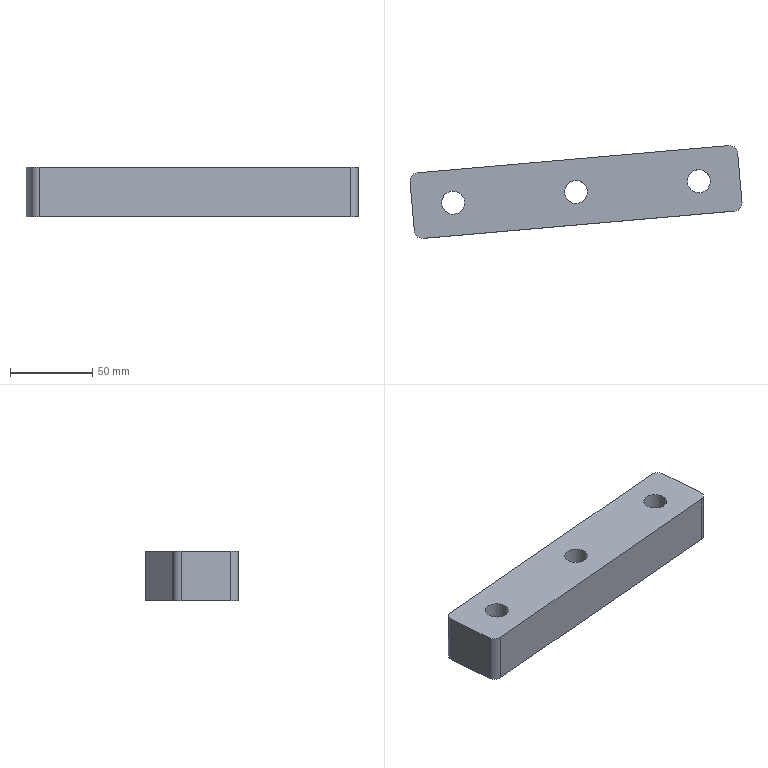Part | NX | features MAIN_BODY 2 | 1 solid | 13 faces | box 201.892 x 56.445 x 30 mm | volume 225502 mm3 | cylinder 7 | plane 6 | commonest cylinder face diameters 10 x4 14 x3
STEP:
#1=CARTESIAN_POINT('',(699.149,728.708,-265.));
#2=VERTEX_POINT('',#1);
#3=CARTESIAN_POINT('',(696.535,758.594,-265.));
#4=VERTEX_POINT('',#3);
#5=CARTESIAN_POINT('',(699.585,723.727,-265.));
#6=DIRECTION('',(-0.08716,0.9962,0.));
#7=VECTOR('',#6,1000.);
#8=LINE('',#5,#7);
#9=EDGE_CURVE('',#2,#4,#8,.T.);
#10=ORIENTED_EDGE('',*,*,#9,.F.);
#11=CARTESIAN_POINT('',(699.149,728.708,-295.));
#12=VERTEX_POINT('',#11);
#13=CARTESIAN_POINT('',(699.149,728.708,-295.));
#14=DIRECTION('',(0.,0.,1.));
#15=VECTOR('',#14,1000.);
#16=LINE('',#13,#15);
#17=EDGE_CURVE('',#2,#12,#16,.F.);
#18=ORIENTED_EDGE('',*,*,#17,.T.);
#19=CARTESIAN_POINT('',(696.535,758.594,-295.));
#20=VERTEX_POINT('',#19);
#21=CARTESIAN_POINT('',(699.585,723.727,-295.));
#22=DIRECTION('',(-0.08716,0.9962,0.));
#23=VECTOR('',#22,1000.);
#24=LINE('',#21,#23);
#25=EDGE_CURVE('',#12,#20,#24,.T.);
#26=ORIENTED_EDGE('',*,*,#25,.T.);
#27=CARTESIAN_POINT('',(696.535,758.594,-295.));
#28=DIRECTION('',(0.,0.,1.));
#29=VECTOR('',#28,1000.);
#30=LINE('',#27,#29);
#31=EDGE_CURVE('',#20,#4,#30,.T.);
#32=ORIENTED_EDGE('',*,*,#31,.T.);
#33=EDGE_LOOP('',(#10,#18,#26,#32));
#34=FACE_BOUND('',#33,.T.);
#35=CARTESIAN_POINT('',(699.585,723.727,-295.));
#36=DIRECTION('',(0.9962,0.08716,0.));
#37=DIRECTION('',(0.08716,-0.9962,0.));
#38=AXIS2_PLACEMENT_3D('',#35,#36,#37);
#39=PLANE('',#38);
#40=ADVANCED_FACE('',(#34),#39,.T.);
#41=CARTESIAN_POINT('',(691.118,763.139,-265.));
#42=VERTEX_POINT('',#41);
#43=CARTESIAN_POINT('',(501.841,746.579,-265.));
#44=VERTEX_POINT('',#43);
#45=CARTESIAN_POINT('',(696.099,763.575,-265.));
#46=DIRECTION('',(-0.9962,-0.08716,0.));
#47=VECTOR('',#46,1000.);
#48=LINE('',#45,#47);
#49=EDGE_CURVE('',#42,#44,#48,.T.);
#50=ORIENTED_EDGE('',*,*,#49,.F.);
#51=CARTESIAN_POINT('',(691.118,763.139,-295.));
#52=VERTEX_POINT('',#51);
#53=CARTESIAN_POINT('',(691.118,763.139,-295.));
#54=DIRECTION('',(0.,0.,1.));
#55=VECTOR('',#54,1000.);
#56=LINE('',#53,#55);
#57=EDGE_CURVE('',#42,#52,#56,.F.);
#58=ORIENTED_EDGE('',*,*,#57,.T.);
#59=CARTESIAN_POINT('',(501.841,746.579,-295.));
#60=VERTEX_POINT('',#59);
#61=CARTESIAN_POINT('',(696.099,763.575,-295.));
#62=DIRECTION('',(-0.9962,-0.08716,0.));
#63=VECTOR('',#62,1000.);
#64=LINE('',#61,#63);
#65=EDGE_CURVE('',#52,#60,#64,.T.);
#66=ORIENTED_EDGE('',*,*,#65,.T.);
#67=CARTESIAN_POINT('',(501.841,746.579,-295.));
#68=DIRECTION('',(0.,0.,1.));
#69=VECTOR('',#68,1000.);
#70=LINE('',#67,#69);
#71=EDGE_CURVE('',#60,#44,#70,.T.);
#72=ORIENTED_EDGE('',*,*,#71,.T.);
#73=EDGE_LOOP('',(#50,#58,#66,#72));
#74=FACE_BOUND('',#73,.T.);
#75=CARTESIAN_POINT('',(696.099,763.575,-295.));
#76=DIRECTION('',(-0.08716,0.9962,0.));
#77=DIRECTION('',(0.9962,0.08716,0.));
#78=AXIS2_PLACEMENT_3D('',#75,#76,#77);
#79=PLANE('',#78);
#80=ADVANCED_FACE('',(#74),#79,.T.);
#81=CARTESIAN_POINT('',(505.327,706.731,-295.));
#82=VERTEX_POINT('',#81);
#83=CARTESIAN_POINT('',(694.604,723.291,-295.));
#84=VERTEX_POINT('',#83);
#85=CARTESIAN_POINT('',(599.966,715.011,-295.));
#86=DIRECTION('',(0.9962,0.08716,0.));
#87=VECTOR('',#86,1000.);
#88=LINE('',#85,#87);
#89=EDGE_CURVE('',#82,#84,#88,.T.);
#90=ORIENTED_EDGE('',*,*,#89,.T.);
#91=CARTESIAN_POINT('',(694.604,723.291,-265.));
#92=VERTEX_POINT('',#91);
#93=CARTESIAN_POINT('',(694.604,723.291,-295.));
#94=DIRECTION('',(0.,0.,1.));
#95=VECTOR('',#94,1000.);
#96=LINE('',#93,#95);
#97=EDGE_CURVE('',#84,#92,#96,.T.);
#98=ORIENTED_EDGE('',*,*,#97,.T.);
#99=CARTESIAN_POINT('',(505.327,706.731,-265.));
#100=VERTEX_POINT('',#99);
#101=CARTESIAN_POINT('',(599.966,715.011,-265.));
#102=DIRECTION('',(0.9962,0.08716,0.));
#103=VECTOR('',#102,1000.);
#104=LINE('',#101,#103);
#105=EDGE_CURVE('',#100,#92,#104,.T.);
#106=ORIENTED_EDGE('',*,*,#105,.F.);
#107=CARTESIAN_POINT('',(505.327,706.731,-295.));
#108=DIRECTION('',(0.,0.,1.));
#109=VECTOR('',#108,1000.);
#110=LINE('',#107,#109);
#111=EDGE_CURVE('',#100,#82,#110,.F.);
#112=ORIENTED_EDGE('',*,*,#111,.T.);
#113=EDGE_LOOP('',(#90,#98,#106,#112));
#114=FACE_BOUND('',#113,.T.);
#115=CARTESIAN_POINT('',(599.966,715.011,-295.));
#116=DIRECTION('',(0.08716,-0.9962,0.));
#117=DIRECTION('',(0.,0.,-1.));
#118=AXIS2_PLACEMENT_3D('',#115,#116,#117);
#119=PLANE('',#118);
#120=ADVANCED_FACE('',(#114),#119,.T.);
#121=ORIENTED_EDGE('',*,*,#25,.F.);
#122=CARTESIAN_POINT('',(694.168,728.272,-295.));
#123=DIRECTION('',(0.,0.,1.));
#124=DIRECTION('',(-0.9962,-0.08716,0.));
#125=AXIS2_PLACEMENT_3D('',#122,#123,#124);
#126=CIRCLE('',#125,5.);
#127=EDGE_CURVE('',#12,#84,#126,.F.);
#128=ORIENTED_EDGE('',*,*,#127,.T.);
#129=ORIENTED_EDGE('',*,*,#89,.F.);
#130=CARTESIAN_POINT('',(499.91,711.277,-295.));
#131=VERTEX_POINT('',#130);
#132=CARTESIAN_POINT('',(504.891,711.712,-295.));
#133=DIRECTION('',(0.,0.,1.));
#134=DIRECTION('',(-0.9962,-0.08716,0.));
#135=AXIS2_PLACEMENT_3D('',#132,#133,#134);
#136=CIRCLE('',#135,5.);
#137=EDGE_CURVE('',#82,#131,#136,.F.);
#138=ORIENTED_EDGE('',*,*,#137,.T.);
#139=CARTESIAN_POINT('',(497.296,741.163,-295.));
#140=VERTEX_POINT('',#139);
#141=CARTESIAN_POINT('',(500.346,706.296,-295.));
#142=DIRECTION('',(-0.08716,0.9962,0.));
#143=VECTOR('',#142,1000.);
#144=LINE('',#141,#143);
#145=EDGE_CURVE('',#131,#140,#144,.T.);
#146=ORIENTED_EDGE('',*,*,#145,.T.);
#147=CARTESIAN_POINT('',(502.277,741.598,-295.));
#148=DIRECTION('',(0.,0.,1.));
#149=DIRECTION('',(-0.9962,-0.08716,0.));
#150=AXIS2_PLACEMENT_3D('',#147,#148,#149);
#151=CIRCLE('',#150,5.);
#152=EDGE_CURVE('',#140,#60,#151,.F.);
#153=ORIENTED_EDGE('',*,*,#152,.T.);
#154=ORIENTED_EDGE('',*,*,#65,.F.);
#155=CARTESIAN_POINT('',(691.554,758.158,-295.));
#156=DIRECTION('',(0.,0.,1.));
#157=DIRECTION('',(-0.9962,-0.08716,0.));
#158=AXIS2_PLACEMENT_3D('',#155,#156,#157);
#159=CIRCLE('',#158,5.);
#160=EDGE_CURVE('',#52,#20,#159,.F.);
#161=ORIENTED_EDGE('',*,*,#160,.T.);
#162=EDGE_LOOP('',(#121,#128,#129,#138,#146,#153,#154,#161));
#163=FACE_BOUND('',#162,.T.);
#164=CARTESIAN_POINT('',(665.964,740.862,-295.));
#165=VERTEX_POINT('',#164);
#166=CARTESIAN_POINT('',(672.937,741.472,-295.));
#167=DIRECTION('',(0.,0.,1.));
#168=DIRECTION('',(-0.9962,-0.08716,0.));
#169=AXIS2_PLACEMENT_3D('',#166,#167,#168);
#170=CIRCLE('',#169,7.);
#171=EDGE_CURVE('',#165,#165,#170,.T.);
#172=ORIENTED_EDGE('',*,*,#171,.T.);
#173=EDGE_LOOP('',(#172));
#174=FACE_BOUND('',#173,.T.);
#175=CARTESIAN_POINT('',(591.249,734.325,-295.));
#176=VERTEX_POINT('',#175);
#177=CARTESIAN_POINT('',(598.223,734.935,-295.));
#178=DIRECTION('',(0.,0.,1.));
#179=DIRECTION('',(-0.9962,-0.08716,0.));
#180=AXIS2_PLACEMENT_3D('',#177,#178,#179);
#181=CIRCLE('',#180,7.);
#182=EDGE_CURVE('',#176,#176,#181,.T.);
#183=ORIENTED_EDGE('',*,*,#182,.T.);
#184=EDGE_LOOP('',(#183));
#185=FACE_BOUND('',#184,.T.);
#186=CARTESIAN_POINT('',(530.481,729.009,-295.));
#187=VERTEX_POINT('',#186);
#188=CARTESIAN_POINT('',(523.508,728.399,-295.));
#189=DIRECTION('',(0.,0.,-1.));
#190=DIRECTION('',(0.9962,0.08716,0.));
#191=AXIS2_PLACEMENT_3D('',#188,#189,#190);
#192=CIRCLE('',#191,7.);
#193=EDGE_CURVE('',#187,#187,#192,.T.);
#194=ORIENTED_EDGE('',*,*,#193,.F.);
#195=EDGE_LOOP('',(#194));
#196=FACE_BOUND('',#195,.T.);
#197=CARTESIAN_POINT('',(696.099,763.575,-295.));
#198=DIRECTION('',(0.,0.,1.));
#199=DIRECTION('',(-0.9962,-0.08716,0.));
#200=AXIS2_PLACEMENT_3D('',#197,#198,#199);
#201=PLANE('',#200);
#202=ADVANCED_FACE('',(#163,#174,#185,#196),#201,.F.);
#203=ORIENTED_EDGE('',*,*,#105,.T.);
#204=CARTESIAN_POINT('',(694.168,728.272,-265.));
#205=DIRECTION('',(0.,0.,1.));
#206=DIRECTION('',(-0.9962,-0.08716,0.));
#207=AXIS2_PLACEMENT_3D('',#204,#205,#206);
#208=CIRCLE('',#207,5.);
#209=EDGE_CURVE('',#92,#2,#208,.T.);
#210=ORIENTED_EDGE('',*,*,#209,.T.);
#211=ORIENTED_EDGE('',*,*,#9,.T.);
#212=CARTESIAN_POINT('',(691.554,758.158,-265.));
#213=DIRECTION('',(0.,0.,1.));
#214=DIRECTION('',(-0.9962,-0.08716,0.));
#215=AXIS2_PLACEMENT_3D('',#212,#213,#214);
#216=CIRCLE('',#215,5.);
#217=EDGE_CURVE('',#4,#42,#216,.T.);
#218=ORIENTED_EDGE('',*,*,#217,.T.);
#219=ORIENTED_EDGE('',*,*,#49,.T.);
#220=CARTESIAN_POINT('',(497.296,741.163,-265.));
#221=VERTEX_POINT('',#220);
#222=CARTESIAN_POINT('',(502.277,741.598,-265.));
#223=DIRECTION('',(0.,0.,1.));
#224=DIRECTION('',(-0.9962,-0.08716,0.));
#225=AXIS2_PLACEMENT_3D('',#222,#223,#224);
#226=CIRCLE('',#225,5.);
#227=EDGE_CURVE('',#44,#221,#226,.T.);
#228=ORIENTED_EDGE('',*,*,#227,.T.);
#229=CARTESIAN_POINT('',(499.91,711.277,-265.));
#230=VERTEX_POINT('',#229);
#231=CARTESIAN_POINT('',(500.346,706.296,-265.));
#232=DIRECTION('',(-0.08716,0.9962,0.));
#233=VECTOR('',#232,1000.);
#234=LINE('',#231,#233);
#235=EDGE_CURVE('',#230,#221,#234,.T.);
#236=ORIENTED_EDGE('',*,*,#235,.F.);
#237=CARTESIAN_POINT('',(504.891,711.712,-265.));
#238=DIRECTION('',(0.,0.,1.));
#239=DIRECTION('',(-0.9962,-0.08716,0.));
#240=AXIS2_PLACEMENT_3D('',#237,#238,#239);
#241=CIRCLE('',#240,5.);
#242=EDGE_CURVE('',#230,#100,#241,.T.);
#243=ORIENTED_EDGE('',*,*,#242,.T.);
#244=EDGE_LOOP('',(#203,#210,#211,#218,#219,#228,#236,#243));
#245=FACE_BOUND('',#244,.T.);
#246=CARTESIAN_POINT('',(591.249,734.325,-265.));
#247=VERTEX_POINT('',#246);
#248=CARTESIAN_POINT('',(598.223,734.935,-265.));
#249=DIRECTION('',(0.,0.,1.));
#250=DIRECTION('',(-0.9962,-0.08716,0.));
#251=AXIS2_PLACEMENT_3D('',#248,#249,#250);
#252=CIRCLE('',#251,7.);
#253=EDGE_CURVE('',#247,#247,#252,.T.);
#254=ORIENTED_EDGE('',*,*,#253,.F.);
#255=EDGE_LOOP('',(#254));
#256=FACE_BOUND('',#255,.T.);
#257=CARTESIAN_POINT('',(665.964,740.862,-265.));
#258=VERTEX_POINT('',#257);
#259=CARTESIAN_POINT('',(672.937,741.472,-265.));
#260=DIRECTION('',(0.,0.,1.));
#261=DIRECTION('',(-0.9962,-0.08716,0.));
#262=AXIS2_PLACEMENT_3D('',#259,#260,#261);
#263=CIRCLE('',#262,7.);
#264=EDGE_CURVE('',#258,#258,#263,.T.);
#265=ORIENTED_EDGE('',*,*,#264,.F.);
#266=EDGE_LOOP('',(#265));
#267=FACE_BOUND('',#266,.T.);
#268=CARTESIAN_POINT('',(530.481,729.009,-265.));
#269=VERTEX_POINT('',#268);
#270=CARTESIAN_POINT('',(523.508,728.399,-265.));
#271=DIRECTION('',(0.,0.,-1.));
#272=DIRECTION('',(0.9962,0.08716,0.));
#273=AXIS2_PLACEMENT_3D('',#270,#271,#272);
#274=CIRCLE('',#273,7.);
#275=EDGE_CURVE('',#269,#269,#274,.T.);
#276=ORIENTED_EDGE('',*,*,#275,.T.);
#277=EDGE_LOOP('',(#276));
#278=FACE_BOUND('',#277,.T.);
#279=CARTESIAN_POINT('',(696.099,763.575,-265.));
#280=DIRECTION('',(0.,0.,1.));
#281=DIRECTION('',(-0.9962,-0.08716,0.));
#282=AXIS2_PLACEMENT_3D('',#279,#280,#281);
#283=PLANE('',#282);
#284=ADVANCED_FACE('',(#245,#256,#267,#278),#283,.T.);
#285=ORIENTED_EDGE('',*,*,#264,.T.);
#286=EDGE_LOOP('',(#285));
#287=FACE_BOUND('',#286,.T.);
#288=ORIENTED_EDGE('',*,*,#171,.F.);
#289=EDGE_LOOP('',(#288));
#290=FACE_BOUND('',#289,.T.);
#291=CARTESIAN_POINT('',(672.937,741.472,-295.));
#292=DIRECTION('',(0.,0.,1.));
#293=DIRECTION('',(-0.9962,-0.08716,0.));
#294=AXIS2_PLACEMENT_3D('',#291,#292,#293);
#295=CYLINDRICAL_SURFACE('',#294,7.);
#296=ADVANCED_FACE('',(#287,#290),#295,.F.);
#297=ORIENTED_EDGE('',*,*,#253,.T.);
#298=EDGE_LOOP('',(#297));
#299=FACE_BOUND('',#298,.T.);
#300=ORIENTED_EDGE('',*,*,#182,.F.);
#301=EDGE_LOOP('',(#300));
#302=FACE_BOUND('',#301,.T.);
#303=CARTESIAN_POINT('',(598.223,734.935,-295.));
#304=DIRECTION('',(0.,0.,1.));
#305=DIRECTION('',(-0.9962,-0.08716,0.));
#306=AXIS2_PLACEMENT_3D('',#303,#304,#305);
#307=CYLINDRICAL_SURFACE('',#306,7.);
#308=ADVANCED_FACE('',(#299,#302),#307,.F.);
#309=ORIENTED_EDGE('',*,*,#145,.F.);
#310=CARTESIAN_POINT('',(499.91,711.277,-295.));
#311=DIRECTION('',(0.,0.,1.));
#312=VECTOR('',#311,1000.);
#313=LINE('',#310,#312);
#314=EDGE_CURVE('',#131,#230,#313,.T.);
#315=ORIENTED_EDGE('',*,*,#314,.T.);
#316=ORIENTED_EDGE('',*,*,#235,.T.);
#317=CARTESIAN_POINT('',(497.296,741.163,-295.));
#318=DIRECTION('',(0.,0.,1.));
#319=VECTOR('',#318,1000.);
#320=LINE('',#317,#319);
#321=EDGE_CURVE('',#221,#140,#320,.F.);
#322=ORIENTED_EDGE('',*,*,#321,.T.);
#323=EDGE_LOOP('',(#309,#315,#316,#322));
#324=FACE_BOUND('',#323,.T.);
#325=CARTESIAN_POINT('',(500.346,706.296,-295.));
#326=DIRECTION('',(-0.9962,-0.08716,0.));
#327=DIRECTION('',(0.08716,-0.9962,0.));
#328=AXIS2_PLACEMENT_3D('',#325,#326,#327);
#329=PLANE('',#328);
#330=ADVANCED_FACE('',(#324),#329,.T.);
#331=ORIENTED_EDGE('',*,*,#275,.F.);
#332=EDGE_LOOP('',(#331));
#333=FACE_BOUND('',#332,.T.);
#334=ORIENTED_EDGE('',*,*,#193,.T.);
#335=EDGE_LOOP('',(#334));
#336=FACE_BOUND('',#335,.T.);
#337=CARTESIAN_POINT('',(523.508,728.399,-295.));
#338=DIRECTION('',(0.,0.,1.));
#339=DIRECTION('',(0.9962,0.08716,0.));
#340=AXIS2_PLACEMENT_3D('',#337,#338,#339);
#341=CYLINDRICAL_SURFACE('',#340,7.);
#342=ADVANCED_FACE('',(#333,#336),#341,.F.);
#343=ORIENTED_EDGE('',*,*,#127,.F.);
#344=ORIENTED_EDGE('',*,*,#17,.F.);
#345=ORIENTED_EDGE('',*,*,#209,.F.);
#346=ORIENTED_EDGE('',*,*,#97,.F.);
#347=EDGE_LOOP('',(#343,#344,#345,#346));
#348=FACE_BOUND('',#347,.T.);
#349=CARTESIAN_POINT('',(694.168,728.272,-295.));
#350=DIRECTION('',(0.,0.,1.));
#351=DIRECTION('',(-0.9962,-0.08716,0.));
#352=AXIS2_PLACEMENT_3D('',#349,#350,#351);
#353=CYLINDRICAL_SURFACE('',#352,5.);
#354=ADVANCED_FACE('',(#348),#353,.T.);
#355=ORIENTED_EDGE('',*,*,#160,.F.);
#356=ORIENTED_EDGE('',*,*,#57,.F.);
#357=ORIENTED_EDGE('',*,*,#217,.F.);
#358=ORIENTED_EDGE('',*,*,#31,.F.);
#359=EDGE_LOOP('',(#355,#356,#357,#358));
#360=FACE_BOUND('',#359,.T.);
#361=CARTESIAN_POINT('',(691.554,758.158,-295.));
#362=DIRECTION('',(0.,0.,1.));
#363=DIRECTION('',(-0.9962,-0.08716,0.));
#364=AXIS2_PLACEMENT_3D('',#361,#362,#363);
#365=CYLINDRICAL_SURFACE('',#364,5.);
#366=ADVANCED_FACE('',(#360),#365,.T.);
#367=ORIENTED_EDGE('',*,*,#137,.F.);
#368=ORIENTED_EDGE('',*,*,#111,.F.);
#369=ORIENTED_EDGE('',*,*,#242,.F.);
#370=ORIENTED_EDGE('',*,*,#314,.F.);
#371=EDGE_LOOP('',(#367,#368,#369,#370));
#372=FACE_BOUND('',#371,.T.);
#373=CARTESIAN_POINT('',(504.891,711.712,-295.));
#374=DIRECTION('',(0.,0.,1.));
#375=DIRECTION('',(-0.9962,-0.08716,0.));
#376=AXIS2_PLACEMENT_3D('',#373,#374,#375);
#377=CYLINDRICAL_SURFACE('',#376,5.);
#378=ADVANCED_FACE('',(#372),#377,.T.);
#379=ORIENTED_EDGE('',*,*,#152,.F.);
#380=ORIENTED_EDGE('',*,*,#321,.F.);
#381=ORIENTED_EDGE('',*,*,#227,.F.);
#382=ORIENTED_EDGE('',*,*,#71,.F.);
#383=EDGE_LOOP('',(#379,#380,#381,#382));
#384=FACE_BOUND('',#383,.T.);
#385=CARTESIAN_POINT('',(502.277,741.598,-295.));
#386=DIRECTION('',(0.,0.,1.));
#387=DIRECTION('',(-0.9962,-0.08716,0.));
#388=AXIS2_PLACEMENT_3D('',#385,#386,#387);
#389=CYLINDRICAL_SURFACE('',#388,5.);
#390=ADVANCED_FACE('',(#384),#389,.T.);
#391=CLOSED_SHELL('',(#40,#80,#120,#202,#284,#296,#308,#330,#342,#354,#366,#378,#390));
#392=MANIFOLD_SOLID_BREP('',#391);
#393=(LENGTH_UNIT()NAMED_UNIT(*)SI_UNIT(.MILLI.,.METRE.));
#394=UNCERTAINTY_MEASURE_WITH_UNIT(LENGTH_MEASURE(0.00001),#393,'','');
#395=(NAMED_UNIT(*)PLANE_ANGLE_UNIT()SI_UNIT($,.RADIAN.));
#396=(NAMED_UNIT(*)SI_UNIT($,.STERADIAN.)SOLID_ANGLE_UNIT());
#397=(GEOMETRIC_REPRESENTATION_CONTEXT(3)GLOBAL_UNCERTAINTY_ASSIGNED_CONTEXT((#394))GLOBAL_UNIT_ASSIGNED_CONTEXT((#393,#395,#396))REPRESENTATION_CONTEXT('',''));
#398=ADVANCED_BREP_SHAPE_REPRESENTATION('',(#392),#397);